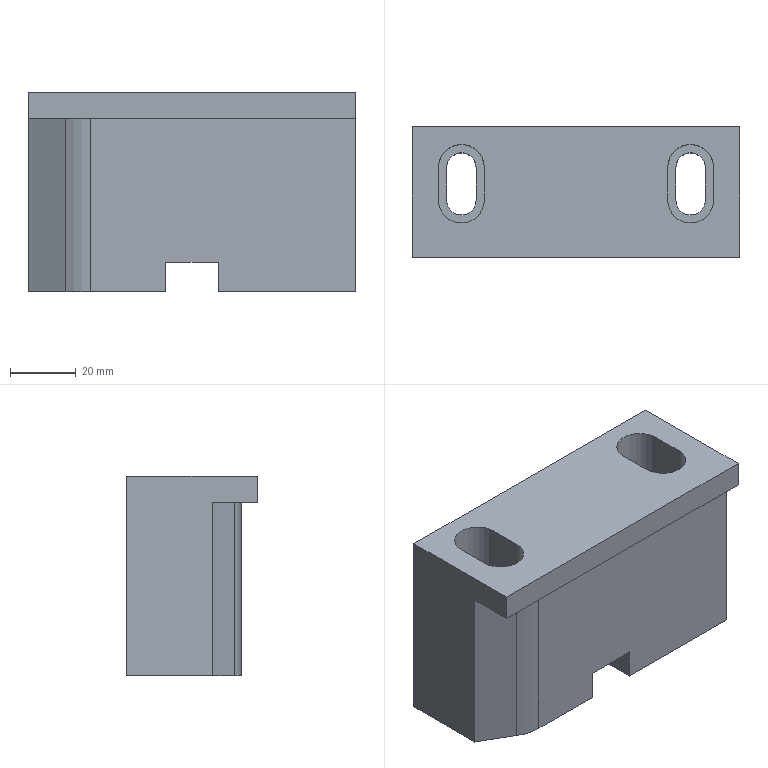Part | NX | features 1605158915 2 | 1 solid | 32 faces | box 100 x 40 x 61 mm | volume 180942 mm3 | plane 23 | cylinder 9 | commonest cylinder face diameters 9 x4 14 x4 30 x1
STEP:
#1=CARTESIAN_POINT('',(-341.,95.35,-2.5));
#2=VERTEX_POINT('',#1);
#3=CARTESIAN_POINT('',(-341.,130.35,-2.5));
#4=VERTEX_POINT('',#3);
#5=CARTESIAN_POINT('',(-341.,113.85,-2.5));
#6=DIRECTION('',(0.,1.,0.));
#7=VECTOR('',#6,1000.);
#8=LINE('',#5,#7);
#9=EDGE_CURVE('',#2,#4,#8,.T.);
#10=ORIENTED_EDGE('',*,*,#9,.F.);
#11=CARTESIAN_POINT('',(-363.981,95.35,-2.5));
#12=VERTEX_POINT('',#11);
#13=CARTESIAN_POINT('',(-333.,95.35,-2.5));
#14=DIRECTION('',(-1.,0.,0.));
#15=VECTOR('',#14,1000.);
#16=LINE('',#13,#15);
#17=EDGE_CURVE('',#2,#12,#16,.T.);
#18=ORIENTED_EDGE('',*,*,#17,.T.);
#19=CARTESIAN_POINT('',(-371.481,97.36,-2.5));
#20=VERTEX_POINT('',#19);
#21=CARTESIAN_POINT('',(-363.981,110.35,-2.5));
#22=DIRECTION('',(0.,0.,1.));
#23=DIRECTION('',(-1.,0.,0.));
#24=AXIS2_PLACEMENT_3D('',#21,#22,#23);
#25=CIRCLE('',#24,15.);
#26=EDGE_CURVE('',#20,#12,#25,.T.);
#27=ORIENTED_EDGE('',*,*,#26,.F.);
#28=CARTESIAN_POINT('',(-383.,104.01,-2.5));
#29=VERTEX_POINT('',#28);
#30=CARTESIAN_POINT('',(-349.761,84.82,-2.5));
#31=DIRECTION('',(-0.866,0.5,0.));
#32=VECTOR('',#31,1000.);
#33=LINE('',#30,#32);
#34=EDGE_CURVE('',#29,#20,#33,.F.);
#35=ORIENTED_EDGE('',*,*,#34,.F.);
#36=CARTESIAN_POINT('',(-383.,130.35,-2.5));
#37=VERTEX_POINT('',#36);
#38=CARTESIAN_POINT('',(-383.,113.85,-2.5));
#39=DIRECTION('',(0.,1.,0.));
#40=VECTOR('',#39,1000.);
#41=LINE('',#38,#40);
#42=EDGE_CURVE('',#29,#37,#41,.T.);
#43=ORIENTED_EDGE('',*,*,#42,.T.);
#44=CARTESIAN_POINT('',(-333.,130.35,-2.5));
#45=DIRECTION('',(1.,0.,0.));
#46=VECTOR('',#45,1000.);
#47=LINE('',#44,#46);
#48=EDGE_CURVE('',#37,#4,#47,.T.);
#49=ORIENTED_EDGE('',*,*,#48,.T.);
#50=EDGE_LOOP('',(#10,#18,#27,#35,#43,#49));
#51=FACE_BOUND('',#50,.T.);
#52=CARTESIAN_POINT('',(-372.5,107.85,-2.5));
#53=VERTEX_POINT('',#52);
#54=CARTESIAN_POINT('',(-363.5,107.85,-2.5));
#55=VERTEX_POINT('',#54);
#56=CARTESIAN_POINT('',(-368.,107.85,-2.5));
#57=DIRECTION('',(0.,0.,1.));
#58=DIRECTION('',(-1.,0.,0.));
#59=AXIS2_PLACEMENT_3D('',#56,#57,#58);
#60=CIRCLE('',#59,4.5);
#61=EDGE_CURVE('',#53,#55,#60,.T.);
#62=ORIENTED_EDGE('',*,*,#61,.T.);
#63=CARTESIAN_POINT('',(-363.5,117.85,-2.5));
#64=VERTEX_POINT('',#63);
#65=CARTESIAN_POINT('',(-363.5,113.85,-2.5));
#66=DIRECTION('',(0.,1.,0.));
#67=VECTOR('',#66,1000.);
#68=LINE('',#65,#67);
#69=EDGE_CURVE('',#55,#64,#68,.T.);
#70=ORIENTED_EDGE('',*,*,#69,.T.);
#71=CARTESIAN_POINT('',(-372.5,117.85,-2.5));
#72=VERTEX_POINT('',#71);
#73=CARTESIAN_POINT('',(-368.,117.85,-2.5));
#74=DIRECTION('',(0.,0.,1.));
#75=DIRECTION('',(-1.,0.,0.));
#76=AXIS2_PLACEMENT_3D('',#73,#74,#75);
#77=CIRCLE('',#76,4.5);
#78=EDGE_CURVE('',#64,#72,#77,.T.);
#79=ORIENTED_EDGE('',*,*,#78,.T.);
#80=CARTESIAN_POINT('',(-372.5,113.85,-2.5));
#81=DIRECTION('',(0.,-1.,0.));
#82=VECTOR('',#81,1000.);
#83=LINE('',#80,#82);
#84=EDGE_CURVE('',#72,#53,#83,.T.);
#85=ORIENTED_EDGE('',*,*,#84,.T.);
#86=EDGE_LOOP('',(#62,#70,#79,#85));
#87=FACE_BOUND('',#86,.T.);
#88=CARTESIAN_POINT('',(-333.,113.85,-2.5));
#89=DIRECTION('',(0.,0.,-1.));
#90=DIRECTION('',(-1.,0.,0.));
#91=AXIS2_PLACEMENT_3D('',#88,#89,#90);
#92=PLANE('',#91);
#93=ADVANCED_FACE('',(#51,#87),#92,.T.);
#94=CARTESIAN_POINT('',(-325.,130.35,-2.5));
#95=VERTEX_POINT('',#94);
#96=CARTESIAN_POINT('',(-325.,95.35,-2.5));
#97=VERTEX_POINT('',#96);
#98=CARTESIAN_POINT('',(-325.,113.85,-2.5));
#99=DIRECTION('',(0.,-1.,0.));
#100=VECTOR('',#99,1000.);
#101=LINE('',#98,#100);
#102=EDGE_CURVE('',#95,#97,#101,.T.);
#103=ORIENTED_EDGE('',*,*,#102,.F.);
#104=CARTESIAN_POINT('',(-283.,130.35,-2.5));
#105=VERTEX_POINT('',#104);
#106=CARTESIAN_POINT('',(-333.,130.35,-2.5));
#107=DIRECTION('',(1.,0.,0.));
#108=VECTOR('',#107,1000.);
#109=LINE('',#106,#108);
#110=EDGE_CURVE('',#95,#105,#109,.T.);
#111=ORIENTED_EDGE('',*,*,#110,.T.);
#112=CARTESIAN_POINT('',(-283.,95.35,-2.5));
#113=VERTEX_POINT('',#112);
#114=CARTESIAN_POINT('',(-283.,-7.65,-2.5));
#115=DIRECTION('',(0.,-1.,0.));
#116=VECTOR('',#115,1000.);
#117=LINE('',#114,#116);
#118=EDGE_CURVE('',#105,#113,#117,.T.);
#119=ORIENTED_EDGE('',*,*,#118,.T.);
#120=CARTESIAN_POINT('',(-333.,95.35,-2.5));
#121=DIRECTION('',(-1.,0.,0.));
#122=VECTOR('',#121,1000.);
#123=LINE('',#120,#122);
#124=EDGE_CURVE('',#113,#97,#123,.T.);
#125=ORIENTED_EDGE('',*,*,#124,.T.);
#126=EDGE_LOOP('',(#103,#111,#119,#125));
#127=FACE_BOUND('',#126,.T.);
#128=CARTESIAN_POINT('',(-302.5,107.85,-2.5));
#129=VERTEX_POINT('',#128);
#130=CARTESIAN_POINT('',(-293.5,107.85,-2.5));
#131=VERTEX_POINT('',#130);
#132=CARTESIAN_POINT('',(-298.,107.85,-2.5));
#133=DIRECTION('',(0.,0.,1.));
#134=DIRECTION('',(-1.,0.,0.));
#135=AXIS2_PLACEMENT_3D('',#132,#133,#134);
#136=CIRCLE('',#135,4.5);
#137=EDGE_CURVE('',#129,#131,#136,.T.);
#138=ORIENTED_EDGE('',*,*,#137,.T.);
#139=CARTESIAN_POINT('',(-293.5,117.85,-2.5));
#140=VERTEX_POINT('',#139);
#141=CARTESIAN_POINT('',(-293.5,113.85,-2.5));
#142=DIRECTION('',(0.,1.,0.));
#143=VECTOR('',#142,1000.);
#144=LINE('',#141,#143);
#145=EDGE_CURVE('',#131,#140,#144,.T.);
#146=ORIENTED_EDGE('',*,*,#145,.T.);
#147=CARTESIAN_POINT('',(-302.5,117.85,-2.5));
#148=VERTEX_POINT('',#147);
#149=CARTESIAN_POINT('',(-298.,117.85,-2.5));
#150=DIRECTION('',(0.,0.,1.));
#151=DIRECTION('',(-1.,0.,0.));
#152=AXIS2_PLACEMENT_3D('',#149,#150,#151);
#153=CIRCLE('',#152,4.5);
#154=EDGE_CURVE('',#140,#148,#153,.T.);
#155=ORIENTED_EDGE('',*,*,#154,.T.);
#156=CARTESIAN_POINT('',(-302.5,113.85,-2.5));
#157=DIRECTION('',(0.,-1.,0.));
#158=VECTOR('',#157,1000.);
#159=LINE('',#156,#158);
#160=EDGE_CURVE('',#148,#129,#159,.T.);
#161=ORIENTED_EDGE('',*,*,#160,.T.);
#162=EDGE_LOOP('',(#138,#146,#155,#161));
#163=FACE_BOUND('',#162,.T.);
#164=CARTESIAN_POINT('',(-333.,113.85,-2.5));
#165=DIRECTION('',(0.,0.,-1.));
#166=DIRECTION('',(-1.,0.,0.));
#167=AXIS2_PLACEMENT_3D('',#164,#165,#166);
#168=PLANE('',#167);
#169=ADVANCED_FACE('',(#127,#163),#168,.T.);
#170=CARTESIAN_POINT('',(-361.,117.85,58.5));
#171=VERTEX_POINT('',#170);
#172=CARTESIAN_POINT('',(-361.,117.85,25.5));
#173=VERTEX_POINT('',#172);
#174=CARTESIAN_POINT('',(-361.,117.85,-2.501));
#175=DIRECTION('',(0.,0.,1.));
#176=VECTOR('',#175,1000.);
#177=LINE('',#174,#176);
#178=EDGE_CURVE('',#171,#173,#177,.F.);
#179=ORIENTED_EDGE('',*,*,#178,.F.);
#180=CARTESIAN_POINT('',(-375.,117.85,58.5));
#181=VERTEX_POINT('',#180);
#182=CARTESIAN_POINT('',(-368.,117.85,58.5));
#183=DIRECTION('',(0.,0.,-1.));
#184=DIRECTION('',(1.,0.,0.));
#185=AXIS2_PLACEMENT_3D('',#182,#183,#184);
#186=CIRCLE('',#185,7.);
#187=EDGE_CURVE('',#181,#171,#186,.T.);
#188=ORIENTED_EDGE('',*,*,#187,.F.);
#189=CARTESIAN_POINT('',(-375.,117.85,25.5));
#190=VERTEX_POINT('',#189);
#191=CARTESIAN_POINT('',(-375.,117.85,-2.501));
#192=DIRECTION('',(0.,0.,1.));
#193=VECTOR('',#192,1000.);
#194=LINE('',#191,#193);
#195=EDGE_CURVE('',#181,#190,#194,.F.);
#196=ORIENTED_EDGE('',*,*,#195,.T.);
#197=CARTESIAN_POINT('',(-368.,117.85,25.5));
#198=DIRECTION('',(0.,0.,-1.));
#199=DIRECTION('',(1.,0.,0.));
#200=AXIS2_PLACEMENT_3D('',#197,#198,#199);
#201=CIRCLE('',#200,7.);
#202=EDGE_CURVE('',#190,#173,#201,.T.);
#203=ORIENTED_EDGE('',*,*,#202,.T.);
#204=EDGE_LOOP('',(#179,#188,#196,#203));
#205=FACE_BOUND('',#204,.T.);
#206=CARTESIAN_POINT('',(-368.,117.85,-2.501));
#207=DIRECTION('',(0.,0.,1.));
#208=DIRECTION('',(1.,0.,0.));
#209=AXIS2_PLACEMENT_3D('',#206,#207,#208);
#210=CYLINDRICAL_SURFACE('',#209,7.);
#211=ADVANCED_FACE('',(#205),#210,.F.);
#212=CARTESIAN_POINT('',(-363.981,95.35,50.5));
#213=VERTEX_POINT('',#212);
#214=CARTESIAN_POINT('',(-283.,95.35,50.5));
#215=VERTEX_POINT('',#214);
#216=CARTESIAN_POINT('',(-333.,95.35,50.5));
#217=DIRECTION('',(1.,0.,0.));
#218=VECTOR('',#217,1000.);
#219=LINE('',#216,#218);
#220=EDGE_CURVE('',#213,#215,#219,.T.);
#221=ORIENTED_EDGE('',*,*,#220,.T.);
#222=CARTESIAN_POINT('',(-283.,90.35,50.5));
#223=VERTEX_POINT('',#222);
#224=CARTESIAN_POINT('',(-283.,-7.65,50.5));
#225=DIRECTION('',(0.,1.,0.));
#226=VECTOR('',#225,1000.);
#227=LINE('',#224,#226);
#228=EDGE_CURVE('',#223,#215,#227,.T.);
#229=ORIENTED_EDGE('',*,*,#228,.F.);
#230=CARTESIAN_POINT('',(-383.,90.35,50.5));
#231=VERTEX_POINT('',#230);
#232=CARTESIAN_POINT('',(-333.,90.35,50.5));
#233=DIRECTION('',(1.,0.,0.));
#234=VECTOR('',#233,1000.);
#235=LINE('',#232,#234);
#236=EDGE_CURVE('',#231,#223,#235,.T.);
#237=ORIENTED_EDGE('',*,*,#236,.F.);
#238=CARTESIAN_POINT('',(-383.,104.01,50.5));
#239=VERTEX_POINT('',#238);
#240=CARTESIAN_POINT('',(-383.,113.85,50.5));
#241=DIRECTION('',(0.,-1.,0.));
#242=VECTOR('',#241,1000.);
#243=LINE('',#240,#242);
#244=EDGE_CURVE('',#239,#231,#243,.T.);
#245=ORIENTED_EDGE('',*,*,#244,.F.);
#246=CARTESIAN_POINT('',(-371.481,97.36,50.5));
#247=VERTEX_POINT('',#246);
#248=CARTESIAN_POINT('',(-379.25,101.845,50.5));
#249=DIRECTION('',(0.866,-0.5,0.));
#250=VECTOR('',#249,1000.);
#251=LINE('',#248,#250);
#252=EDGE_CURVE('',#247,#239,#251,.F.);
#253=ORIENTED_EDGE('',*,*,#252,.F.);
#254=CARTESIAN_POINT('',(-363.981,110.35,50.5));
#255=DIRECTION('',(0.,0.,-1.));
#256=DIRECTION('',(1.,0.,0.));
#257=AXIS2_PLACEMENT_3D('',#254,#255,#256);
#258=CIRCLE('',#257,15.);
#259=EDGE_CURVE('',#213,#247,#258,.T.);
#260=ORIENTED_EDGE('',*,*,#259,.F.);
#261=EDGE_LOOP('',(#221,#229,#237,#245,#253,#260));
#262=FACE_BOUND('',#261,.T.);
#263=CARTESIAN_POINT('',(-383.,95.35,50.5));
#264=DIRECTION('',(0.,0.,1.));
#265=DIRECTION('',(1.,0.,0.));
#266=AXIS2_PLACEMENT_3D('',#263,#264,#265);
#267=PLANE('',#266);
#268=ADVANCED_FACE('',(#262),#267,.F.);
#269=CARTESIAN_POINT('',(-341.,130.35,6.5));
#270=VERTEX_POINT('',#269);
#271=CARTESIAN_POINT('',(-325.,130.35,6.5));
#272=VERTEX_POINT('',#271);
#273=CARTESIAN_POINT('',(-333.,130.35,6.5));
#274=DIRECTION('',(-1.,0.,0.));
#275=VECTOR('',#274,1000.);
#276=LINE('',#273,#275);
#277=EDGE_CURVE('',#270,#272,#276,.F.);
#278=ORIENTED_EDGE('',*,*,#277,.F.);
#279=CARTESIAN_POINT('',(-341.,130.35,-2.5));
#280=DIRECTION('',(0.,0.,1.));
#281=VECTOR('',#280,1000.);
#282=LINE('',#279,#281);
#283=EDGE_CURVE('',#4,#270,#282,.T.);
#284=ORIENTED_EDGE('',*,*,#283,.F.);
#285=ORIENTED_EDGE('',*,*,#48,.F.);
#286=CARTESIAN_POINT('',(-383.,130.35,58.5));
#287=VERTEX_POINT('',#286);
#288=CARTESIAN_POINT('',(-383.,130.35,-2.5));
#289=DIRECTION('',(0.,0.,1.));
#290=VECTOR('',#289,1000.);
#291=LINE('',#288,#290);
#292=EDGE_CURVE('',#37,#287,#291,.T.);
#293=ORIENTED_EDGE('',*,*,#292,.T.);
#294=CARTESIAN_POINT('',(-283.,130.35,58.5));
#295=VERTEX_POINT('',#294);
#296=CARTESIAN_POINT('',(-333.,130.35,58.5));
#297=DIRECTION('',(-1.,0.,0.));
#298=VECTOR('',#297,1000.);
#299=LINE('',#296,#298);
#300=EDGE_CURVE('',#295,#287,#299,.T.);
#301=ORIENTED_EDGE('',*,*,#300,.F.);
#302=CARTESIAN_POINT('',(-283.,130.35,-2.5));
#303=DIRECTION('',(0.,0.,1.));
#304=VECTOR('',#303,1000.);
#305=LINE('',#302,#304);
#306=EDGE_CURVE('',#105,#295,#305,.T.);
#307=ORIENTED_EDGE('',*,*,#306,.F.);
#308=ORIENTED_EDGE('',*,*,#110,.F.);
#309=CARTESIAN_POINT('',(-325.,130.35,2.5));
#310=DIRECTION('',(0.,0.,1.));
#311=VECTOR('',#310,1000.);
#312=LINE('',#309,#311);
#313=EDGE_CURVE('',#95,#272,#312,.T.);
#314=ORIENTED_EDGE('',*,*,#313,.T.);
#315=EDGE_LOOP('',(#278,#284,#285,#293,#301,#307,#308,#314));
#316=FACE_BOUND('',#315,.T.);
#317=CARTESIAN_POINT('',(-333.,130.35,-2.5));
#318=DIRECTION('',(0.,1.,0.));
#319=DIRECTION('',(0.,0.,-1.));
#320=AXIS2_PLACEMENT_3D('',#317,#318,#319);
#321=PLANE('',#320);
#322=ADVANCED_FACE('',(#316),#321,.T.);
#323=ORIENTED_EDGE('',*,*,#244,.T.);
#324=CARTESIAN_POINT('',(-383.,90.35,58.5));
#325=VERTEX_POINT('',#324);
#326=CARTESIAN_POINT('',(-383.,90.35,15.5));
#327=DIRECTION('',(0.,0.,1.));
#328=VECTOR('',#327,1000.);
#329=LINE('',#326,#328);
#330=EDGE_CURVE('',#231,#325,#329,.T.);
#331=ORIENTED_EDGE('',*,*,#330,.T.);
#332=CARTESIAN_POINT('',(-383.,113.85,58.5));
#333=DIRECTION('',(0.,-1.,0.));
#334=VECTOR('',#333,1000.);
#335=LINE('',#332,#334);
#336=EDGE_CURVE('',#287,#325,#335,.T.);
#337=ORIENTED_EDGE('',*,*,#336,.F.);
#338=ORIENTED_EDGE('',*,*,#292,.F.);
#339=ORIENTED_EDGE('',*,*,#42,.F.);
#340=CARTESIAN_POINT('',(-383.,104.01,-2.5));
#341=DIRECTION('',(0.,0.,-1.));
#342=VECTOR('',#341,1000.);
#343=LINE('',#340,#342);
#344=EDGE_CURVE('',#239,#29,#343,.T.);
#345=ORIENTED_EDGE('',*,*,#344,.F.);
#346=EDGE_LOOP('',(#323,#331,#337,#338,#339,#345));
#347=FACE_BOUND('',#346,.T.);
#348=CARTESIAN_POINT('',(-383.,113.85,-2.5));
#349=DIRECTION('',(-1.,0.,0.));
#350=DIRECTION('',(0.,0.,1.));
#351=AXIS2_PLACEMENT_3D('',#348,#349,#350);
#352=PLANE('',#351);
#353=ADVANCED_FACE('',(#347),#352,.T.);
#354=ORIENTED_EDGE('',*,*,#236,.T.);
#355=CARTESIAN_POINT('',(-283.,90.35,58.5));
#356=VERTEX_POINT('',#355);
#357=CARTESIAN_POINT('',(-283.,90.35,-17.5));
#358=DIRECTION('',(0.,0.,1.));
#359=VECTOR('',#358,1000.);
#360=LINE('',#357,#359);
#361=EDGE_CURVE('',#223,#356,#360,.T.);
#362=ORIENTED_EDGE('',*,*,#361,.T.);
#363=CARTESIAN_POINT('',(-333.,90.35,58.5));
#364=DIRECTION('',(1.,0.,0.));
#365=VECTOR('',#364,1000.);
#366=LINE('',#363,#365);
#367=EDGE_CURVE('',#325,#356,#366,.T.);
#368=ORIENTED_EDGE('',*,*,#367,.F.);
#369=ORIENTED_EDGE('',*,*,#330,.F.);
#370=EDGE_LOOP('',(#354,#362,#368,#369));
#371=FACE_BOUND('',#370,.T.);
#372=CARTESIAN_POINT('',(-333.,90.35,15.5));
#373=DIRECTION('',(0.,-1.,0.));
#374=DIRECTION('',(0.,0.,1.));
#375=AXIS2_PLACEMENT_3D('',#372,#373,#374);
#376=PLANE('',#375);
#377=ADVANCED_FACE('',(#371),#376,.T.);
#378=ORIENTED_EDGE('',*,*,#228,.T.);
#379=CARTESIAN_POINT('',(-283.,95.35,-35.5));
#380=DIRECTION('',(0.,0.,1.));
#381=VECTOR('',#380,1000.);
#382=LINE('',#379,#381);
#383=EDGE_CURVE('',#113,#215,#382,.T.);
#384=ORIENTED_EDGE('',*,*,#383,.F.);
#385=ORIENTED_EDGE('',*,*,#118,.F.);
#386=ORIENTED_EDGE('',*,*,#306,.T.);
#387=CARTESIAN_POINT('',(-283.,-7.65,58.5));
#388=DIRECTION('',(0.,1.,0.));
#389=VECTOR('',#388,1000.);
#390=LINE('',#387,#389);
#391=EDGE_CURVE('',#356,#295,#390,.T.);
#392=ORIENTED_EDGE('',*,*,#391,.F.);
#393=ORIENTED_EDGE('',*,*,#361,.F.);
#394=EDGE_LOOP('',(#378,#384,#385,#386,#392,#393));
#395=FACE_BOUND('',#394,.T.);
#396=CARTESIAN_POINT('',(-283.,-7.65,-35.5));
#397=DIRECTION('',(1.,0.,0.));
#398=DIRECTION('',(0.,0.,-1.));
#399=AXIS2_PLACEMENT_3D('',#396,#397,#398);
#400=PLANE('',#399);
#401=ADVANCED_FACE('',(#395),#400,.T.);
#402=CARTESIAN_POINT('',(-341.,95.35,6.5));
#403=VERTEX_POINT('',#402);
#404=CARTESIAN_POINT('',(-341.,95.35,-2.5));
#405=DIRECTION('',(0.,0.,-1.));
#406=VECTOR('',#405,1000.);
#407=LINE('',#404,#406);
#408=EDGE_CURVE('',#403,#2,#407,.T.);
#409=ORIENTED_EDGE('',*,*,#408,.F.);
#410=CARTESIAN_POINT('',(-325.,95.35,6.5));
#411=VERTEX_POINT('',#410);
#412=CARTESIAN_POINT('',(-333.,95.35,6.5));
#413=DIRECTION('',(1.,0.,0.));
#414=VECTOR('',#413,1000.);
#415=LINE('',#412,#414);
#416=EDGE_CURVE('',#411,#403,#415,.F.);
#417=ORIENTED_EDGE('',*,*,#416,.F.);
#418=CARTESIAN_POINT('',(-325.,95.35,-2.5));
#419=DIRECTION('',(0.,0.,1.));
#420=VECTOR('',#419,1000.);
#421=LINE('',#418,#420);
#422=EDGE_CURVE('',#97,#411,#421,.T.);
#423=ORIENTED_EDGE('',*,*,#422,.F.);
#424=ORIENTED_EDGE('',*,*,#124,.F.);
#425=ORIENTED_EDGE('',*,*,#383,.T.);
#426=ORIENTED_EDGE('',*,*,#220,.F.);
#427=CARTESIAN_POINT('',(-363.981,95.35,-2.5));
#428=DIRECTION('',(0.,0.,-1.));
#429=VECTOR('',#428,1000.);
#430=LINE('',#427,#429);
#431=EDGE_CURVE('',#12,#213,#430,.F.);
#432=ORIENTED_EDGE('',*,*,#431,.F.);
#433=ORIENTED_EDGE('',*,*,#17,.F.);
#434=EDGE_LOOP('',(#409,#417,#423,#424,#425,#426,#432,#433));
#435=FACE_BOUND('',#434,.T.);
#436=CARTESIAN_POINT('',(-333.,95.35,-2.5));
#437=DIRECTION('',(0.,-1.,0.));
#438=DIRECTION('',(0.,0.,1.));
#439=AXIS2_PLACEMENT_3D('',#436,#437,#438);
#440=PLANE('',#439);
#441=ADVANCED_FACE('',(#435),#440,.T.);
#442=ORIENTED_EDGE('',*,*,#252,.T.);
#443=ORIENTED_EDGE('',*,*,#344,.T.);
#444=ORIENTED_EDGE('',*,*,#34,.T.);
#445=CARTESIAN_POINT('',(-371.481,97.36,-2.5));
#446=DIRECTION('',(0.,0.,1.));
#447=VECTOR('',#446,1000.);
#448=LINE('',#445,#447);
#449=EDGE_CURVE('',#247,#20,#448,.F.);
#450=ORIENTED_EDGE('',*,*,#449,.F.);
#451=EDGE_LOOP('',(#442,#443,#444,#450));
#452=FACE_BOUND('',#451,.T.);
#453=CARTESIAN_POINT('',(-368.,95.35,-2.5));
#454=DIRECTION('',(0.5,0.866,0.));
#455=DIRECTION('',(0.866,-0.5,0.));
#456=AXIS2_PLACEMENT_3D('',#453,#454,#455);
#457=PLANE('',#456);
#458=ADVANCED_FACE('',(#452),#457,.F.);
#459=ORIENTED_EDGE('',*,*,#26,.T.);
#460=ORIENTED_EDGE('',*,*,#431,.T.);
#461=ORIENTED_EDGE('',*,*,#259,.T.);
#462=ORIENTED_EDGE('',*,*,#449,.T.);
#463=EDGE_LOOP('',(#459,#460,#461,#462));
#464=FACE_BOUND('',#463,.T.);
#465=CARTESIAN_POINT('',(-363.981,110.35,-2.5));
#466=DIRECTION('',(0.,0.,-1.));
#467=DIRECTION('',(-1.,0.,0.));
#468=AXIS2_PLACEMENT_3D('',#465,#466,#467);
#469=CYLINDRICAL_SURFACE('',#468,15.);
#470=ADVANCED_FACE('',(#464),#469,.T.);
#471=ORIENTED_EDGE('',*,*,#195,.F.);
#472=CARTESIAN_POINT('',(-375.,107.85,58.5));
#473=VERTEX_POINT('',#472);
#474=CARTESIAN_POINT('',(-375.,113.85,58.5));
#475=DIRECTION('',(0.,1.,0.));
#476=VECTOR('',#475,1000.);
#477=LINE('',#474,#476);
#478=EDGE_CURVE('',#473,#181,#477,.T.);
#479=ORIENTED_EDGE('',*,*,#478,.F.);
#480=CARTESIAN_POINT('',(-375.,107.85,25.5));
#481=VERTEX_POINT('',#480);
#482=CARTESIAN_POINT('',(-375.,107.85,-2.501));
#483=DIRECTION('',(0.,0.,1.));
#484=VECTOR('',#483,1000.);
#485=LINE('',#482,#484);
#486=EDGE_CURVE('',#481,#473,#485,.T.);
#487=ORIENTED_EDGE('',*,*,#486,.F.);
#488=CARTESIAN_POINT('',(-375.,113.85,25.5));
#489=DIRECTION('',(0.,1.,0.));
#490=VECTOR('',#489,1000.);
#491=LINE('',#488,#490);
#492=EDGE_CURVE('',#481,#190,#491,.T.);
#493=ORIENTED_EDGE('',*,*,#492,.T.);
#494=EDGE_LOOP('',(#471,#479,#487,#493));
#495=FACE_BOUND('',#494,.T.);
#496=CARTESIAN_POINT('',(-375.,120.35,-2.501));
#497=DIRECTION('',(-1.,0.,0.));
#498=DIRECTION('',(0.,0.,1.));
#499=AXIS2_PLACEMENT_3D('',#496,#497,#498);
#500=PLANE('',#499);
#501=ADVANCED_FACE('',(#495),#500,.F.);
#502=CARTESIAN_POINT('',(-361.,107.85,25.5));
#503=VERTEX_POINT('',#502);
#504=CARTESIAN_POINT('',(-361.,107.85,58.5));
#505=VERTEX_POINT('',#504);
#506=CARTESIAN_POINT('',(-361.,107.85,-2.501));
#507=DIRECTION('',(0.,0.,1.));
#508=VECTOR('',#507,1000.);
#509=LINE('',#506,#508);
#510=EDGE_CURVE('',#503,#505,#509,.T.);
#511=ORIENTED_EDGE('',*,*,#510,.T.);
#512=CARTESIAN_POINT('',(-361.,113.85,58.5));
#513=DIRECTION('',(0.,-1.,0.));
#514=VECTOR('',#513,1000.);
#515=LINE('',#512,#514);
#516=EDGE_CURVE('',#171,#505,#515,.T.);
#517=ORIENTED_EDGE('',*,*,#516,.F.);
#518=ORIENTED_EDGE('',*,*,#178,.T.);
#519=CARTESIAN_POINT('',(-361.,113.85,25.5));
#520=DIRECTION('',(0.,-1.,0.));
#521=VECTOR('',#520,1000.);
#522=LINE('',#519,#521);
#523=EDGE_CURVE('',#173,#503,#522,.T.);
#524=ORIENTED_EDGE('',*,*,#523,.T.);
#525=EDGE_LOOP('',(#511,#517,#518,#524));
#526=FACE_BOUND('',#525,.T.);
#527=CARTESIAN_POINT('',(-361.,105.35,-2.501));
#528=DIRECTION('',(1.,0.,0.));
#529=DIRECTION('',(0.,0.,-1.));
#530=AXIS2_PLACEMENT_3D('',#527,#528,#529);
#531=PLANE('',#530);
#532=ADVANCED_FACE('',(#526),#531,.F.);
#533=ORIENTED_EDGE('',*,*,#486,.T.);
#534=CARTESIAN_POINT('',(-368.,107.85,58.5));
#535=DIRECTION('',(0.,0.,-1.));
#536=DIRECTION('',(1.,0.,0.));
#537=AXIS2_PLACEMENT_3D('',#534,#535,#536);
#538=CIRCLE('',#537,7.);
#539=EDGE_CURVE('',#505,#473,#538,.T.);
#540=ORIENTED_EDGE('',*,*,#539,.F.);
#541=ORIENTED_EDGE('',*,*,#510,.F.);
#542=CARTESIAN_POINT('',(-368.,107.85,25.5));
#543=DIRECTION('',(0.,0.,-1.));
#544=DIRECTION('',(1.,0.,0.));
#545=AXIS2_PLACEMENT_3D('',#542,#543,#544);
#546=CIRCLE('',#545,7.);
#547=EDGE_CURVE('',#503,#481,#546,.T.);
#548=ORIENTED_EDGE('',*,*,#547,.T.);
#549=EDGE_LOOP('',(#533,#540,#541,#548));
#550=FACE_BOUND('',#549,.T.);
#551=CARTESIAN_POINT('',(-368.,107.85,-2.501));
#552=DIRECTION('',(0.,0.,1.));
#553=DIRECTION('',(1.,0.,0.));
#554=AXIS2_PLACEMENT_3D('',#551,#552,#553);
#555=CYLINDRICAL_SURFACE('',#554,7.);
#556=ADVANCED_FACE('',(#550),#555,.F.);
#557=CARTESIAN_POINT('',(-363.5,107.85,25.5));
#558=VERTEX_POINT('',#557);
#559=CARTESIAN_POINT('',(-372.5,107.85,25.5));
#560=VERTEX_POINT('',#559);
#561=CARTESIAN_POINT('',(-368.,107.85,25.5));
#562=DIRECTION('',(0.,0.,-1.));
#563=DIRECTION('',(1.,0.,0.));
#564=AXIS2_PLACEMENT_3D('',#561,#562,#563);
#565=CIRCLE('',#564,4.5);
#566=EDGE_CURVE('',#558,#560,#565,.T.);
#567=ORIENTED_EDGE('',*,*,#566,.F.);
#568=CARTESIAN_POINT('',(-363.5,107.85,-2.501));
#569=DIRECTION('',(0.,0.,1.));
#570=VECTOR('',#569,1000.);
#571=LINE('',#568,#570);
#572=EDGE_CURVE('',#55,#558,#571,.T.);
#573=ORIENTED_EDGE('',*,*,#572,.F.);
#574=ORIENTED_EDGE('',*,*,#61,.F.);
#575=CARTESIAN_POINT('',(-372.5,107.85,-2.501));
#576=DIRECTION('',(0.,0.,1.));
#577=VECTOR('',#576,1000.);
#578=LINE('',#575,#577);
#579=EDGE_CURVE('',#53,#560,#578,.T.);
#580=ORIENTED_EDGE('',*,*,#579,.T.);
#581=EDGE_LOOP('',(#567,#573,#574,#580));
#582=FACE_BOUND('',#581,.T.);
#583=CARTESIAN_POINT('',(-368.,107.85,-2.501));
#584=DIRECTION('',(0.,0.,1.));
#585=DIRECTION('',(1.,0.,0.));
#586=AXIS2_PLACEMENT_3D('',#583,#584,#585);
#587=CYLINDRICAL_SURFACE('',#586,4.5);
#588=ADVANCED_FACE('',(#582),#587,.F.);
#589=ORIENTED_EDGE('',*,*,#566,.T.);
#590=CARTESIAN_POINT('',(-372.5,117.85,25.5));
#591=VERTEX_POINT('',#590);
#592=CARTESIAN_POINT('',(-372.5,113.85,25.5));
#593=DIRECTION('',(0.,1.,0.));
#594=VECTOR('',#593,1000.);
#595=LINE('',#592,#594);
#596=EDGE_CURVE('',#560,#591,#595,.T.);
#597=ORIENTED_EDGE('',*,*,#596,.T.);
#598=CARTESIAN_POINT('',(-363.5,117.85,25.5));
#599=VERTEX_POINT('',#598);
#600=CARTESIAN_POINT('',(-368.,117.85,25.5));
#601=DIRECTION('',(0.,0.,-1.));
#602=DIRECTION('',(1.,0.,0.));
#603=AXIS2_PLACEMENT_3D('',#600,#601,#602);
#604=CIRCLE('',#603,4.5);
#605=EDGE_CURVE('',#591,#599,#604,.T.);
#606=ORIENTED_EDGE('',*,*,#605,.T.);
#607=CARTESIAN_POINT('',(-363.5,113.85,25.5));
#608=DIRECTION('',(0.,-1.,0.));
#609=VECTOR('',#608,1000.);
#610=LINE('',#607,#609);
#611=EDGE_CURVE('',#599,#558,#610,.T.);
#612=ORIENTED_EDGE('',*,*,#611,.T.);
#613=EDGE_LOOP('',(#589,#597,#606,#612));
#614=FACE_BOUND('',#613,.T.);
#615=ORIENTED_EDGE('',*,*,#202,.F.);
#616=ORIENTED_EDGE('',*,*,#492,.F.);
#617=ORIENTED_EDGE('',*,*,#547,.F.);
#618=ORIENTED_EDGE('',*,*,#523,.F.);
#619=EDGE_LOOP('',(#615,#616,#617,#618));
#620=FACE_BOUND('',#619,.T.);
#621=CARTESIAN_POINT('',(-333.,113.85,25.5));
#622=DIRECTION('',(0.,0.,1.));
#623=DIRECTION('',(1.,0.,0.));
#624=AXIS2_PLACEMENT_3D('',#621,#622,#623);
#625=PLANE('',#624);
#626=ADVANCED_FACE('',(#614,#620),#625,.T.);
#627=ORIENTED_EDGE('',*,*,#596,.F.);
#628=ORIENTED_EDGE('',*,*,#579,.F.);
#629=ORIENTED_EDGE('',*,*,#84,.F.);
#630=CARTESIAN_POINT('',(-372.5,117.85,-2.501));
#631=DIRECTION('',(0.,0.,1.));
#632=VECTOR('',#631,1000.);
#633=LINE('',#630,#632);
#634=EDGE_CURVE('',#72,#591,#633,.T.);
#635=ORIENTED_EDGE('',*,*,#634,.T.);
#636=EDGE_LOOP('',(#627,#628,#629,#635));
#637=FACE_BOUND('',#636,.T.);
#638=CARTESIAN_POINT('',(-372.5,120.35,-2.501));
#639=DIRECTION('',(-1.,0.,0.));
#640=DIRECTION('',(0.,0.,1.));
#641=AXIS2_PLACEMENT_3D('',#638,#639,#640);
#642=PLANE('',#641);
#643=ADVANCED_FACE('',(#637),#642,.F.);
#644=ORIENTED_EDGE('',*,*,#78,.F.);
#645=CARTESIAN_POINT('',(-363.5,117.85,-2.501));
#646=DIRECTION('',(0.,0.,1.));
#647=VECTOR('',#646,1000.);
#648=LINE('',#645,#647);
#649=EDGE_CURVE('',#64,#599,#648,.T.);
#650=ORIENTED_EDGE('',*,*,#649,.T.);
#651=ORIENTED_EDGE('',*,*,#605,.F.);
#652=ORIENTED_EDGE('',*,*,#634,.F.);
#653=EDGE_LOOP('',(#644,#650,#651,#652));
#654=FACE_BOUND('',#653,.T.);
#655=CARTESIAN_POINT('',(-368.,117.85,-2.501));
#656=DIRECTION('',(0.,0.,1.));
#657=DIRECTION('',(1.,0.,0.));
#658=AXIS2_PLACEMENT_3D('',#655,#656,#657);
#659=CYLINDRICAL_SURFACE('',#658,4.5);
#660=ADVANCED_FACE('',(#654),#659,.F.);
#661=ORIENTED_EDGE('',*,*,#611,.F.);
#662=ORIENTED_EDGE('',*,*,#649,.F.);
#663=ORIENTED_EDGE('',*,*,#69,.F.);
#664=ORIENTED_EDGE('',*,*,#572,.T.);
#665=EDGE_LOOP('',(#661,#662,#663,#664));
#666=FACE_BOUND('',#665,.T.);
#667=CARTESIAN_POINT('',(-363.5,105.35,-2.501));
#668=DIRECTION('',(1.,0.,0.));
#669=DIRECTION('',(0.,0.,-1.));
#670=AXIS2_PLACEMENT_3D('',#667,#668,#669);
#671=PLANE('',#670);
#672=ADVANCED_FACE('',(#666),#671,.F.);
#673=CARTESIAN_POINT('',(-291.,117.85,25.5));
#674=VERTEX_POINT('',#673);
#675=CARTESIAN_POINT('',(-305.,117.85,25.5));
#676=VERTEX_POINT('',#675);
#677=CARTESIAN_POINT('',(-298.,117.85,25.5));
#678=DIRECTION('',(0.,0.,-1.));
#679=DIRECTION('',(1.,0.,0.));
#680=AXIS2_PLACEMENT_3D('',#677,#678,#679);
#681=CIRCLE('',#680,7.);
#682=EDGE_CURVE('',#674,#676,#681,.F.);
#683=ORIENTED_EDGE('',*,*,#682,.F.);
#684=CARTESIAN_POINT('',(-291.,117.85,58.5));
#685=VERTEX_POINT('',#684);
#686=CARTESIAN_POINT('',(-291.,117.85,-2.501));
#687=DIRECTION('',(0.,0.,1.));
#688=VECTOR('',#687,1000.);
#689=LINE('',#686,#688);
#690=EDGE_CURVE('',#674,#685,#689,.T.);
#691=ORIENTED_EDGE('',*,*,#690,.T.);
#692=CARTESIAN_POINT('',(-305.,117.85,58.5));
#693=VERTEX_POINT('',#692);
#694=CARTESIAN_POINT('',(-298.,117.85,58.5));
#695=DIRECTION('',(0.,0.,-1.));
#696=DIRECTION('',(1.,0.,0.));
#697=AXIS2_PLACEMENT_3D('',#694,#695,#696);
#698=CIRCLE('',#697,7.);
#699=EDGE_CURVE('',#685,#693,#698,.F.);
#700=ORIENTED_EDGE('',*,*,#699,.T.);
#701=CARTESIAN_POINT('',(-305.,117.85,-2.501));
#702=DIRECTION('',(0.,0.,1.));
#703=VECTOR('',#702,1000.);
#704=LINE('',#701,#703);
#705=EDGE_CURVE('',#676,#693,#704,.T.);
#706=ORIENTED_EDGE('',*,*,#705,.F.);
#707=EDGE_LOOP('',(#683,#691,#700,#706));
#708=FACE_BOUND('',#707,.T.);
#709=CARTESIAN_POINT('',(-298.,117.85,-2.501));
#710=DIRECTION('',(0.,0.,1.));
#711=DIRECTION('',(1.,0.,0.));
#712=AXIS2_PLACEMENT_3D('',#709,#710,#711);
#713=CYLINDRICAL_SURFACE('',#712,7.);
#714=ADVANCED_FACE('',(#708),#713,.F.);
#715=CARTESIAN_POINT('',(-305.,107.85,25.5));
#716=VERTEX_POINT('',#715);
#717=CARTESIAN_POINT('',(-305.,113.85,25.5));
#718=DIRECTION('',(0.,-1.,0.));
#719=VECTOR('',#718,1000.);
#720=LINE('',#717,#719);
#721=EDGE_CURVE('',#676,#716,#720,.T.);
#722=ORIENTED_EDGE('',*,*,#721,.F.);
#723=ORIENTED_EDGE('',*,*,#705,.T.);
#724=CARTESIAN_POINT('',(-305.,107.85,58.5));
#725=VERTEX_POINT('',#724);
#726=CARTESIAN_POINT('',(-305.,113.85,58.5));
#727=DIRECTION('',(0.,-1.,0.));
#728=VECTOR('',#727,1000.);
#729=LINE('',#726,#728);
#730=EDGE_CURVE('',#693,#725,#729,.T.);
#731=ORIENTED_EDGE('',*,*,#730,.T.);
#732=CARTESIAN_POINT('',(-305.,107.85,-2.501));
#733=DIRECTION('',(0.,0.,1.));
#734=VECTOR('',#733,1000.);
#735=LINE('',#732,#734);
#736=EDGE_CURVE('',#716,#725,#735,.T.);
#737=ORIENTED_EDGE('',*,*,#736,.F.);
#738=EDGE_LOOP('',(#722,#723,#731,#737));
#739=FACE_BOUND('',#738,.T.);
#740=CARTESIAN_POINT('',(-305.,107.85,-2.501));
#741=DIRECTION('',(1.,0.,0.));
#742=DIRECTION('',(0.,0.,-1.));
#743=AXIS2_PLACEMENT_3D('',#740,#741,#742);
#744=PLANE('',#743);
#745=ADVANCED_FACE('',(#739),#744,.T.);
#746=CARTESIAN_POINT('',(-291.,107.85,25.5));
#747=VERTEX_POINT('',#746);
#748=CARTESIAN_POINT('',(-298.,107.85,25.5));
#749=DIRECTION('',(0.,0.,-1.));
#750=DIRECTION('',(1.,0.,0.));
#751=AXIS2_PLACEMENT_3D('',#748,#749,#750);
#752=CIRCLE('',#751,7.);
#753=EDGE_CURVE('',#716,#747,#752,.F.);
#754=ORIENTED_EDGE('',*,*,#753,.F.);
#755=ORIENTED_EDGE('',*,*,#736,.T.);
#756=CARTESIAN_POINT('',(-291.,107.85,58.5));
#757=VERTEX_POINT('',#756);
#758=CARTESIAN_POINT('',(-298.,107.85,58.5));
#759=DIRECTION('',(0.,0.,-1.));
#760=DIRECTION('',(1.,0.,0.));
#761=AXIS2_PLACEMENT_3D('',#758,#759,#760);
#762=CIRCLE('',#761,7.);
#763=EDGE_CURVE('',#725,#757,#762,.F.);
#764=ORIENTED_EDGE('',*,*,#763,.T.);
#765=CARTESIAN_POINT('',(-291.,107.85,-2.501));
#766=DIRECTION('',(0.,0.,1.));
#767=VECTOR('',#766,1000.);
#768=LINE('',#765,#767);
#769=EDGE_CURVE('',#747,#757,#768,.T.);
#770=ORIENTED_EDGE('',*,*,#769,.F.);
#771=EDGE_LOOP('',(#754,#755,#764,#770));
#772=FACE_BOUND('',#771,.T.);
#773=CARTESIAN_POINT('',(-298.,107.85,-2.501));
#774=DIRECTION('',(0.,0.,1.));
#775=DIRECTION('',(1.,0.,0.));
#776=AXIS2_PLACEMENT_3D('',#773,#774,#775);
#777=CYLINDRICAL_SURFACE('',#776,7.);
#778=ADVANCED_FACE('',(#772),#777,.F.);
#779=CARTESIAN_POINT('',(-291.,113.85,25.5));
#780=DIRECTION('',(0.,1.,0.));
#781=VECTOR('',#780,1000.);
#782=LINE('',#779,#781);
#783=EDGE_CURVE('',#747,#674,#782,.T.);
#784=ORIENTED_EDGE('',*,*,#783,.F.);
#785=ORIENTED_EDGE('',*,*,#769,.T.);
#786=CARTESIAN_POINT('',(-291.,113.85,58.5));
#787=DIRECTION('',(0.,1.,0.));
#788=VECTOR('',#787,1000.);
#789=LINE('',#786,#788);
#790=EDGE_CURVE('',#757,#685,#789,.T.);
#791=ORIENTED_EDGE('',*,*,#790,.T.);
#792=ORIENTED_EDGE('',*,*,#690,.F.);
#793=EDGE_LOOP('',(#784,#785,#791,#792));
#794=FACE_BOUND('',#793,.T.);
#795=CARTESIAN_POINT('',(-291.,117.85,-2.501));
#796=DIRECTION('',(-1.,0.,0.));
#797=DIRECTION('',(0.,0.,1.));
#798=AXIS2_PLACEMENT_3D('',#795,#796,#797);
#799=PLANE('',#798);
#800=ADVANCED_FACE('',(#794),#799,.T.);
#801=CARTESIAN_POINT('',(-293.5,117.85,25.5));
#802=VERTEX_POINT('',#801);
#803=CARTESIAN_POINT('',(-293.5,107.85,25.5));
#804=VERTEX_POINT('',#803);
#805=CARTESIAN_POINT('',(-293.5,113.85,25.5));
#806=DIRECTION('',(0.,-1.,0.));
#807=VECTOR('',#806,1000.);
#808=LINE('',#805,#807);
#809=EDGE_CURVE('',#802,#804,#808,.T.);
#810=ORIENTED_EDGE('',*,*,#809,.F.);
#811=CARTESIAN_POINT('',(-293.5,117.85,-2.501));
#812=DIRECTION('',(0.,0.,1.));
#813=VECTOR('',#812,1000.);
#814=LINE('',#811,#813);
#815=EDGE_CURVE('',#140,#802,#814,.T.);
#816=ORIENTED_EDGE('',*,*,#815,.F.);
#817=ORIENTED_EDGE('',*,*,#145,.F.);
#818=CARTESIAN_POINT('',(-293.5,107.85,-2.501));
#819=DIRECTION('',(0.,0.,1.));
#820=VECTOR('',#819,1000.);
#821=LINE('',#818,#820);
#822=EDGE_CURVE('',#131,#804,#821,.T.);
#823=ORIENTED_EDGE('',*,*,#822,.T.);
#824=EDGE_LOOP('',(#810,#816,#817,#823));
#825=FACE_BOUND('',#824,.T.);
#826=CARTESIAN_POINT('',(-293.5,107.85,-2.501));
#827=DIRECTION('',(1.,0.,0.));
#828=DIRECTION('',(0.,0.,-1.));
#829=AXIS2_PLACEMENT_3D('',#826,#827,#828);
#830=PLANE('',#829);
#831=ADVANCED_FACE('',(#825),#830,.F.);
#832=CARTESIAN_POINT('',(-302.5,117.85,25.5));
#833=VERTEX_POINT('',#832);
#834=CARTESIAN_POINT('',(-298.,117.85,25.5));
#835=DIRECTION('',(0.,0.,-1.));
#836=DIRECTION('',(1.,0.,0.));
#837=AXIS2_PLACEMENT_3D('',#834,#835,#836);
#838=CIRCLE('',#837,4.5);
#839=EDGE_CURVE('',#833,#802,#838,.T.);
#840=ORIENTED_EDGE('',*,*,#839,.F.);
#841=CARTESIAN_POINT('',(-302.5,117.85,-2.501));
#842=DIRECTION('',(0.,0.,1.));
#843=VECTOR('',#842,1000.);
#844=LINE('',#841,#843);
#845=EDGE_CURVE('',#148,#833,#844,.T.);
#846=ORIENTED_EDGE('',*,*,#845,.F.);
#847=ORIENTED_EDGE('',*,*,#154,.F.);
#848=ORIENTED_EDGE('',*,*,#815,.T.);
#849=EDGE_LOOP('',(#840,#846,#847,#848));
#850=FACE_BOUND('',#849,.T.);
#851=CARTESIAN_POINT('',(-298.,117.85,-2.501));
#852=DIRECTION('',(0.,0.,1.));
#853=DIRECTION('',(1.,0.,0.));
#854=AXIS2_PLACEMENT_3D('',#851,#852,#853);
#855=CYLINDRICAL_SURFACE('',#854,4.5);
#856=ADVANCED_FACE('',(#850),#855,.F.);
#857=CARTESIAN_POINT('',(-302.5,107.85,25.5));
#858=VERTEX_POINT('',#857);
#859=CARTESIAN_POINT('',(-302.5,113.85,25.5));
#860=DIRECTION('',(0.,1.,0.));
#861=VECTOR('',#860,1000.);
#862=LINE('',#859,#861);
#863=EDGE_CURVE('',#858,#833,#862,.T.);
#864=ORIENTED_EDGE('',*,*,#863,.F.);
#865=CARTESIAN_POINT('',(-302.5,107.85,-2.501));
#866=DIRECTION('',(0.,0.,1.));
#867=VECTOR('',#866,1000.);
#868=LINE('',#865,#867);
#869=EDGE_CURVE('',#129,#858,#868,.T.);
#870=ORIENTED_EDGE('',*,*,#869,.F.);
#871=ORIENTED_EDGE('',*,*,#160,.F.);
#872=ORIENTED_EDGE('',*,*,#845,.T.);
#873=EDGE_LOOP('',(#864,#870,#871,#872));
#874=FACE_BOUND('',#873,.T.);
#875=CARTESIAN_POINT('',(-302.5,117.85,-2.501));
#876=DIRECTION('',(-1.,0.,0.));
#877=DIRECTION('',(0.,0.,1.));
#878=AXIS2_PLACEMENT_3D('',#875,#876,#877);
#879=PLANE('',#878);
#880=ADVANCED_FACE('',(#874),#879,.F.);
#881=ORIENTED_EDGE('',*,*,#682,.T.);
#882=ORIENTED_EDGE('',*,*,#721,.T.);
#883=ORIENTED_EDGE('',*,*,#753,.T.);
#884=ORIENTED_EDGE('',*,*,#783,.T.);
#885=EDGE_LOOP('',(#881,#882,#883,#884));
#886=FACE_BOUND('',#885,.T.);
#887=CARTESIAN_POINT('',(-298.,107.85,25.5));
#888=DIRECTION('',(0.,0.,-1.));
#889=DIRECTION('',(1.,0.,0.));
#890=AXIS2_PLACEMENT_3D('',#887,#888,#889);
#891=CIRCLE('',#890,4.5);
#892=EDGE_CURVE('',#804,#858,#891,.T.);
#893=ORIENTED_EDGE('',*,*,#892,.T.);
#894=ORIENTED_EDGE('',*,*,#863,.T.);
#895=ORIENTED_EDGE('',*,*,#839,.T.);
#896=ORIENTED_EDGE('',*,*,#809,.T.);
#897=EDGE_LOOP('',(#893,#894,#895,#896));
#898=FACE_BOUND('',#897,.T.);
#899=CARTESIAN_POINT('',(-333.,113.85,25.5));
#900=DIRECTION('',(0.,0.,1.));
#901=DIRECTION('',(1.,0.,0.));
#902=AXIS2_PLACEMENT_3D('',#899,#900,#901);
#903=PLANE('',#902);
#904=ADVANCED_FACE('',(#886,#898),#903,.T.);
#905=ORIENTED_EDGE('',*,*,#892,.F.);
#906=ORIENTED_EDGE('',*,*,#822,.F.);
#907=ORIENTED_EDGE('',*,*,#137,.F.);
#908=ORIENTED_EDGE('',*,*,#869,.T.);
#909=EDGE_LOOP('',(#905,#906,#907,#908));
#910=FACE_BOUND('',#909,.T.);
#911=CARTESIAN_POINT('',(-298.,107.85,-2.501));
#912=DIRECTION('',(0.,0.,1.));
#913=DIRECTION('',(1.,0.,0.));
#914=AXIS2_PLACEMENT_3D('',#911,#912,#913);
#915=CYLINDRICAL_SURFACE('',#914,4.5);
#916=ADVANCED_FACE('',(#910),#915,.F.);
#917=ORIENTED_EDGE('',*,*,#790,.F.);
#918=ORIENTED_EDGE('',*,*,#763,.F.);
#919=ORIENTED_EDGE('',*,*,#730,.F.);
#920=ORIENTED_EDGE('',*,*,#699,.F.);
#921=EDGE_LOOP('',(#917,#918,#919,#920));
#922=FACE_BOUND('',#921,.T.);
#923=ORIENTED_EDGE('',*,*,#539,.T.);
#924=ORIENTED_EDGE('',*,*,#478,.T.);
#925=ORIENTED_EDGE('',*,*,#187,.T.);
#926=ORIENTED_EDGE('',*,*,#516,.T.);
#927=EDGE_LOOP('',(#923,#924,#925,#926));
#928=FACE_BOUND('',#927,.T.);
#929=ORIENTED_EDGE('',*,*,#300,.T.);
#930=ORIENTED_EDGE('',*,*,#336,.T.);
#931=ORIENTED_EDGE('',*,*,#367,.T.);
#932=ORIENTED_EDGE('',*,*,#391,.T.);
#933=EDGE_LOOP('',(#929,#930,#931,#932));
#934=FACE_BOUND('',#933,.T.);
#935=CARTESIAN_POINT('',(-333.,113.85,58.5));
#936=DIRECTION('',(0.,0.,1.));
#937=DIRECTION('',(1.,0.,0.));
#938=AXIS2_PLACEMENT_3D('',#935,#936,#937);
#939=PLANE('',#938);
#940=ADVANCED_FACE('',(#922,#928,#934),#939,.T.);
#941=ORIENTED_EDGE('',*,*,#9,.T.);
#942=ORIENTED_EDGE('',*,*,#283,.T.);
#943=CARTESIAN_POINT('',(-341.,110.35,6.5));
#944=DIRECTION('',(0.,1.,0.));
#945=VECTOR('',#944,1000.);
#946=LINE('',#943,#945);
#947=EDGE_CURVE('',#403,#270,#946,.T.);
#948=ORIENTED_EDGE('',*,*,#947,.F.);
#949=ORIENTED_EDGE('',*,*,#408,.T.);
#950=EDGE_LOOP('',(#941,#942,#948,#949));
#951=FACE_BOUND('',#950,.T.);
#952=CARTESIAN_POINT('',(-341.,110.35,2.5));
#953=DIRECTION('',(-1.,0.,0.));
#954=DIRECTION('',(0.,0.,-1.));
#955=AXIS2_PLACEMENT_3D('',#952,#953,#954);
#956=PLANE('',#955);
#957=ADVANCED_FACE('',(#951),#956,.F.);
#958=ORIENTED_EDGE('',*,*,#277,.T.);
#959=CARTESIAN_POINT('',(-325.,110.35,6.5));
#960=DIRECTION('',(0.,-1.,0.));
#961=VECTOR('',#960,1000.);
#962=LINE('',#959,#961);
#963=EDGE_CURVE('',#272,#411,#962,.T.);
#964=ORIENTED_EDGE('',*,*,#963,.T.);
#965=ORIENTED_EDGE('',*,*,#416,.T.);
#966=ORIENTED_EDGE('',*,*,#947,.T.);
#967=EDGE_LOOP('',(#958,#964,#965,#966));
#968=FACE_BOUND('',#967,.T.);
#969=CARTESIAN_POINT('',(-325.,110.35,6.5));
#970=DIRECTION('',(0.,0.,-1.));
#971=DIRECTION('',(1.,0.,0.));
#972=AXIS2_PLACEMENT_3D('',#969,#970,#971);
#973=PLANE('',#972);
#974=ADVANCED_FACE('',(#968),#973,.T.);
#975=ORIENTED_EDGE('',*,*,#102,.T.);
#976=ORIENTED_EDGE('',*,*,#422,.T.);
#977=ORIENTED_EDGE('',*,*,#963,.F.);
#978=ORIENTED_EDGE('',*,*,#313,.F.);
#979=EDGE_LOOP('',(#975,#976,#977,#978));
#980=FACE_BOUND('',#979,.T.);
#981=CARTESIAN_POINT('',(-325.,110.35,2.5));
#982=DIRECTION('',(1.,0.,0.));
#983=DIRECTION('',(0.,0.,1.));
#984=AXIS2_PLACEMENT_3D('',#981,#982,#983);
#985=PLANE('',#984);
#986=ADVANCED_FACE('',(#980),#985,.F.);
#987=CLOSED_SHELL('',(#93,#169,#211,#268,#322,#353,#377,#401,#441,#458,#470,#501,#532,#556,#588,#626,#643,#660,#672,#714,#745,#778,#800,#831,#856,#880,#904,#916,#940,#957,#974,#986));
#988=MANIFOLD_SOLID_BREP('',#987);
#989=(LENGTH_UNIT()NAMED_UNIT(*)SI_UNIT(.MILLI.,.METRE.));
#990=UNCERTAINTY_MEASURE_WITH_UNIT(LENGTH_MEASURE(0.00001),#989,'','');
#991=(NAMED_UNIT(*)PLANE_ANGLE_UNIT()SI_UNIT($,.RADIAN.));
#992=(NAMED_UNIT(*)SI_UNIT($,.STERADIAN.)SOLID_ANGLE_UNIT());
#993=(GEOMETRIC_REPRESENTATION_CONTEXT(3)GLOBAL_UNCERTAINTY_ASSIGNED_CONTEXT((#990))GLOBAL_UNIT_ASSIGNED_CONTEXT((#989,#991,#992))REPRESENTATION_CONTEXT('',''));
#994=ADVANCED_BREP_SHAPE_REPRESENTATION('',(#988),#993);